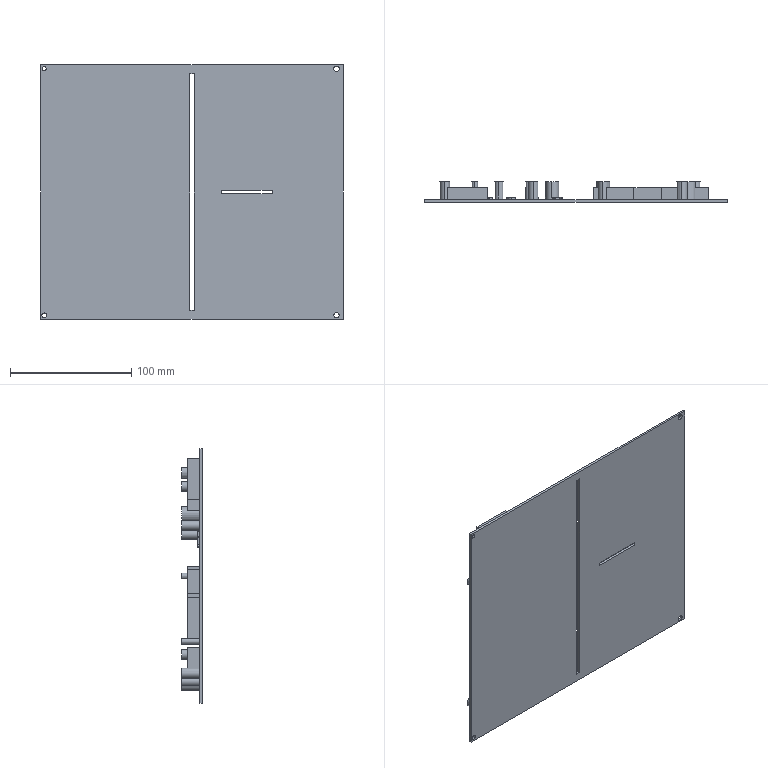Part | STEP file | PCB board | 1 solid | 186 faces | box 250 x 17 x 210 mm | volume 172722 mm3 | plane 116 | spline 38 | cylinder 32 | commonest cylinder face diameters 10.88 x4 3.309 x2 3.847 x2 4.352 x2 4.486 x2 4.725 x2